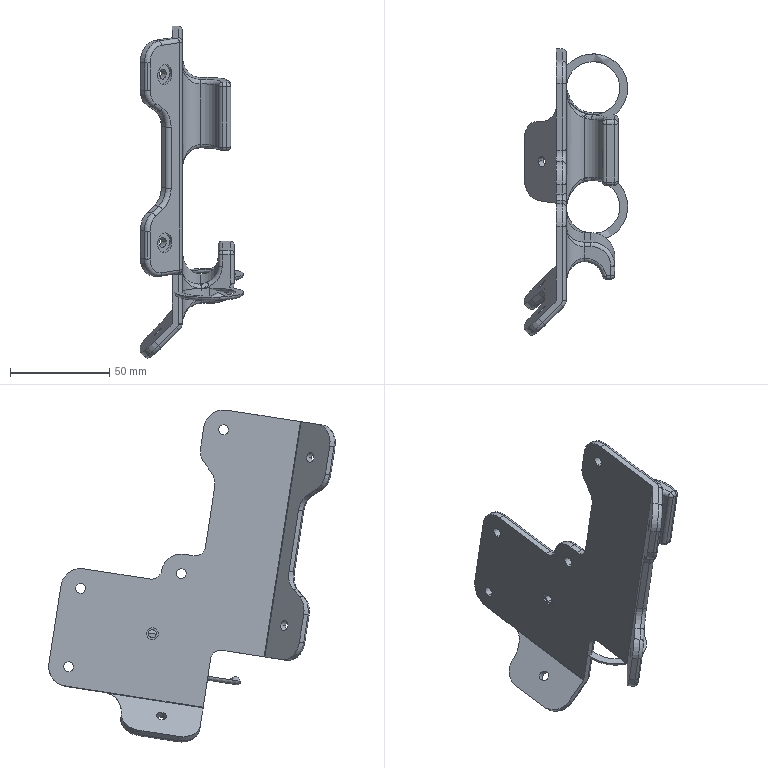Part | SolidWorks | features BaseBody 1 | 1 solid | 222 faces | box 52.213 x 144.491 x 167.396 mm | volume 88752 mm3 | cylinder 110 | plane 44 | torus 40 | spline 16 | sphere 12 | commonest cylinder face diameters 4 x46 10 x19 20 x16 5 x14 18 x8 1 x2